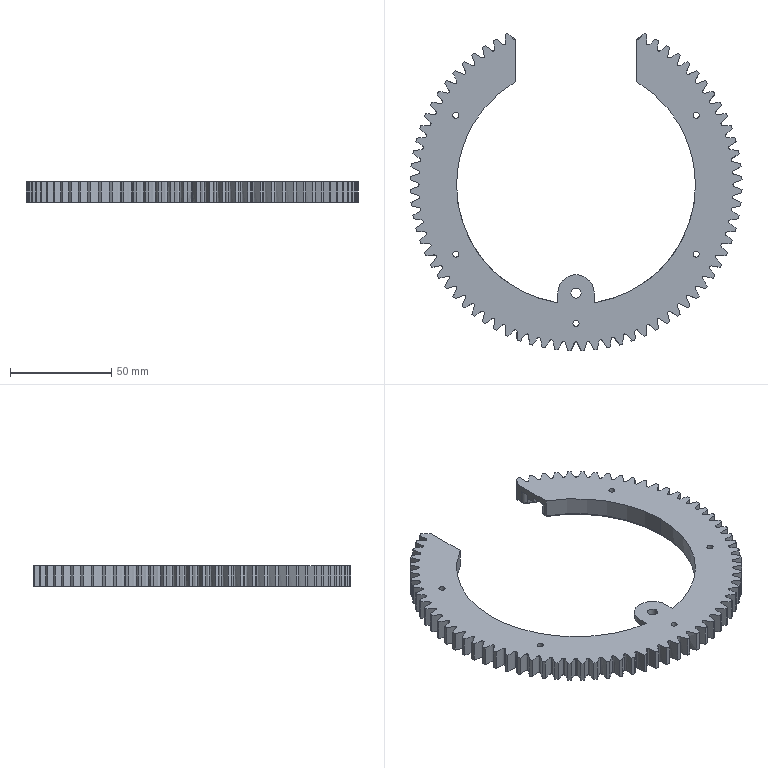Part | STEP file | Packing half-gear | 1 solid | 369 faces | box 163.929 x 156.763 x 10 mm | volume 60681 mm3 | cylinder 196 | spline 140 | plane 20 | torus 13 | commonest cylinder face diameters 154.998 x70 164 x70 7 x11 3 x10 133 x7 141 x7